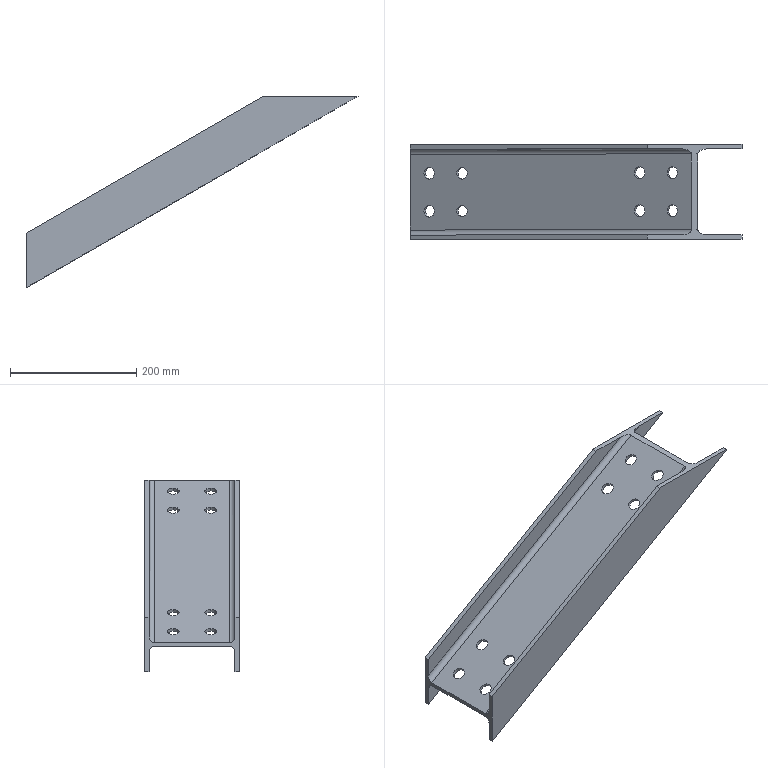Part | STEP file | 粉仓Diagonal Brace梁6-1_Default<As Machined> | 1 solid | 34 faces | box 525.333 x 150 x 303.301 mm | volume 916827 mm3 | cylinder 20 | plane 14 | commonest cylinder face diameters 19 x16 16 x4